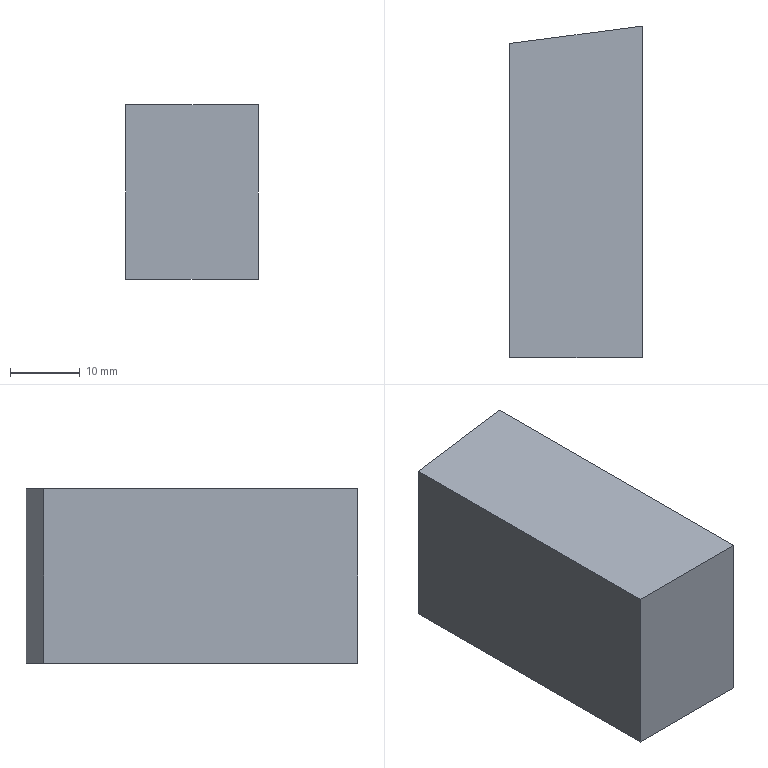Part | SolidWorks | features Extrusion 1 | 1 solid | 6 faces | box 19 x 47.5 x 25 mm | volume 21969 mm3 | plane 6
STEP:
#1=CARTESIAN_POINT('',(0.,45.,0.));
#2=VERTEX_POINT('',#1);
#3=CARTESIAN_POINT('',(0.,0.,0.));
#4=VERTEX_POINT('',#3);
#5=CARTESIAN_POINT('',(0.,0.,0.));
#6=DIRECTION('',(0.,-1.,0.));
#7=VECTOR('',#6,1000.);
#8=LINE('',#5,#7);
#9=EDGE_CURVE('',#2,#4,#8,.T.);
#10=ORIENTED_EDGE('',*,*,#9,.T.);
#11=CARTESIAN_POINT('',(0.,0.,25.));
#12=VERTEX_POINT('',#11);
#13=CARTESIAN_POINT('',(0.,0.,25.));
#14=DIRECTION('',(0.,0.,-1.));
#15=VECTOR('',#14,1000.);
#16=LINE('',#13,#15);
#17=EDGE_CURVE('',#12,#4,#16,.T.);
#18=ORIENTED_EDGE('',*,*,#17,.F.);
#19=CARTESIAN_POINT('',(0.,45.,25.));
#20=VERTEX_POINT('',#19);
#21=CARTESIAN_POINT('',(0.,0.,25.));
#22=DIRECTION('',(0.,-1.,0.));
#23=VECTOR('',#22,1000.);
#24=LINE('',#21,#23);
#25=EDGE_CURVE('',#20,#12,#24,.T.);
#26=ORIENTED_EDGE('',*,*,#25,.F.);
#27=CARTESIAN_POINT('',(0.,45.,25.));
#28=DIRECTION('',(0.,0.,-1.));
#29=VECTOR('',#28,1000.);
#30=LINE('',#27,#29);
#31=EDGE_CURVE('',#20,#2,#30,.T.);
#32=ORIENTED_EDGE('',*,*,#31,.T.);
#33=EDGE_LOOP('',(#10,#18,#26,#32));
#34=FACE_OUTER_BOUND('',#33,.T.);
#35=CARTESIAN_POINT('',(0.,0.,25.));
#36=DIRECTION('',(1.,0.,0.));
#37=DIRECTION('',(0.,1.,0.));
#38=AXIS2_PLACEMENT_3D('',#35,#36,#37);
#39=PLANE('',#38);
#40=ADVANCED_FACE('',(#34),#39,.F.);
#41=CARTESIAN_POINT('',(19.,0.,0.));
#42=VERTEX_POINT('',#41);
#43=CARTESIAN_POINT('',(0.,0.,0.));
#44=DIRECTION('',(1.,0.,0.));
#45=VECTOR('',#44,1000.);
#46=LINE('',#43,#45);
#47=EDGE_CURVE('',#4,#42,#46,.T.);
#48=ORIENTED_EDGE('',*,*,#47,.T.);
#49=CARTESIAN_POINT('',(19.,0.,25.));
#50=VERTEX_POINT('',#49);
#51=CARTESIAN_POINT('',(19.,0.,25.));
#52=DIRECTION('',(0.,0.,-1.));
#53=VECTOR('',#52,1000.);
#54=LINE('',#51,#53);
#55=EDGE_CURVE('',#50,#42,#54,.T.);
#56=ORIENTED_EDGE('',*,*,#55,.F.);
#57=CARTESIAN_POINT('',(0.,0.,25.));
#58=DIRECTION('',(1.,0.,0.));
#59=VECTOR('',#58,1000.);
#60=LINE('',#57,#59);
#61=EDGE_CURVE('',#12,#50,#60,.T.);
#62=ORIENTED_EDGE('',*,*,#61,.F.);
#63=ORIENTED_EDGE('',*,*,#17,.T.);
#64=EDGE_LOOP('',(#48,#56,#62,#63));
#65=FACE_OUTER_BOUND('',#64,.T.);
#66=CARTESIAN_POINT('',(0.,0.,25.));
#67=DIRECTION('',(0.,1.,0.));
#68=DIRECTION('',(0.,0.,1.));
#69=AXIS2_PLACEMENT_3D('',#66,#67,#68);
#70=PLANE('',#69);
#71=ADVANCED_FACE('',(#65),#70,.F.);
#72=CARTESIAN_POINT('',(19.,47.5,0.));
#73=VERTEX_POINT('',#72);
#74=CARTESIAN_POINT('',(19.,0.,0.));
#75=DIRECTION('',(0.,1.,0.));
#76=VECTOR('',#75,1000.);
#77=LINE('',#74,#76);
#78=EDGE_CURVE('',#42,#73,#77,.T.);
#79=ORIENTED_EDGE('',*,*,#78,.T.);
#80=CARTESIAN_POINT('',(19.,47.5,25.));
#81=VERTEX_POINT('',#80);
#82=CARTESIAN_POINT('',(19.,47.5,25.));
#83=DIRECTION('',(0.,0.,-1.));
#84=VECTOR('',#83,1000.);
#85=LINE('',#82,#84);
#86=EDGE_CURVE('',#81,#73,#85,.T.);
#87=ORIENTED_EDGE('',*,*,#86,.F.);
#88=CARTESIAN_POINT('',(19.,0.,25.));
#89=DIRECTION('',(0.,1.,0.));
#90=VECTOR('',#89,1000.);
#91=LINE('',#88,#90);
#92=EDGE_CURVE('',#50,#81,#91,.T.);
#93=ORIENTED_EDGE('',*,*,#92,.F.);
#94=ORIENTED_EDGE('',*,*,#55,.T.);
#95=EDGE_LOOP('',(#79,#87,#93,#94));
#96=FACE_OUTER_BOUND('',#95,.T.);
#97=CARTESIAN_POINT('',(19.,0.,25.));
#98=DIRECTION('',(-1.,0.,0.));
#99=DIRECTION('',(0.,-1.,0.));
#100=AXIS2_PLACEMENT_3D('',#97,#98,#99);
#101=PLANE('',#100);
#102=ADVANCED_FACE('',(#96),#101,.F.);
#103=CARTESIAN_POINT('',(0.,45.,0.));
#104=DIRECTION('',(-0.9915,-0.1305,0.));
#105=VECTOR('',#104,1000.);
#106=LINE('',#103,#105);
#107=EDGE_CURVE('',#73,#2,#106,.T.);
#108=ORIENTED_EDGE('',*,*,#107,.T.);
#109=ORIENTED_EDGE('',*,*,#31,.F.);
#110=CARTESIAN_POINT('',(0.,45.,25.));
#111=DIRECTION('',(-0.9915,-0.1305,0.));
#112=VECTOR('',#111,1000.);
#113=LINE('',#110,#112);
#114=EDGE_CURVE('',#81,#20,#113,.T.);
#115=ORIENTED_EDGE('',*,*,#114,.F.);
#116=ORIENTED_EDGE('',*,*,#86,.T.);
#117=EDGE_LOOP('',(#108,#109,#115,#116));
#118=FACE_OUTER_BOUND('',#117,.T.);
#119=CARTESIAN_POINT('',(0.,45.,25.));
#120=DIRECTION('',(0.1305,-0.9915,0.));
#121=DIRECTION('',(0.9915,0.1305,0.));
#122=AXIS2_PLACEMENT_3D('',#119,#120,#121);
#123=PLANE('',#122);
#124=ADVANCED_FACE('',(#118),#123,.F.);
#125=ORIENTED_EDGE('',*,*,#25,.T.);
#126=ORIENTED_EDGE('',*,*,#61,.T.);
#127=ORIENTED_EDGE('',*,*,#92,.T.);
#128=ORIENTED_EDGE('',*,*,#114,.T.);
#129=EDGE_LOOP('',(#125,#126,#127,#128));
#130=FACE_OUTER_BOUND('',#129,.T.);
#131=CARTESIAN_POINT('',(0.,0.,25.));
#132=DIRECTION('',(0.,0.,-1.));
#133=DIRECTION('',(-1.,0.,0.));
#134=AXIS2_PLACEMENT_3D('',#131,#132,#133);
#135=PLANE('',#134);
#136=ADVANCED_FACE('',(#130),#135,.F.);
#137=ORIENTED_EDGE('',*,*,#9,.F.);
#138=ORIENTED_EDGE('',*,*,#107,.F.);
#139=ORIENTED_EDGE('',*,*,#78,.F.);
#140=ORIENTED_EDGE('',*,*,#47,.F.);
#141=EDGE_LOOP('',(#137,#138,#139,#140));
#142=FACE_OUTER_BOUND('',#141,.T.);
#143=CARTESIAN_POINT('',(0.,0.,0.));
#144=DIRECTION('',(0.,0.,-1.));
#145=DIRECTION('',(-1.,0.,0.));
#146=AXIS2_PLACEMENT_3D('',#143,#144,#145);
#147=PLANE('',#146);
#148=ADVANCED_FACE('',(#142),#147,.T.);
#149=CLOSED_SHELL('',(#40,#71,#102,#124,#136,#148));
#150=MANIFOLD_SOLID_BREP('',#149);
#151=CARTESIAN_POINT('',(0.,0.,0.));
#152=DIRECTION('',(0.,0.,1.));
#153=DIRECTION('',(1.,0.,0.));
#154=AXIS2_PLACEMENT_3D('',#151,#152,#153);
#155=(LENGTH_UNIT()NAMED_UNIT(*)SI_UNIT(.MILLI.,.METRE.));
#156=UNCERTAINTY_MEASURE_WITH_UNIT(LENGTH_MEASURE(0.00001),#155,'','');
#157=(NAMED_UNIT(*)PLANE_ANGLE_UNIT()SI_UNIT($,.RADIAN.));
#158=(NAMED_UNIT(*)SI_UNIT($,.STERADIAN.)SOLID_ANGLE_UNIT());
#159=(GEOMETRIC_REPRESENTATION_CONTEXT(3)GLOBAL_UNCERTAINTY_ASSIGNED_CONTEXT((#156))GLOBAL_UNIT_ASSIGNED_CONTEXT((#155,#157,#158))REPRESENTATION_CONTEXT('',''));
#160=ADVANCED_BREP_SHAPE_REPRESENTATION('',(#150,#154),#159);